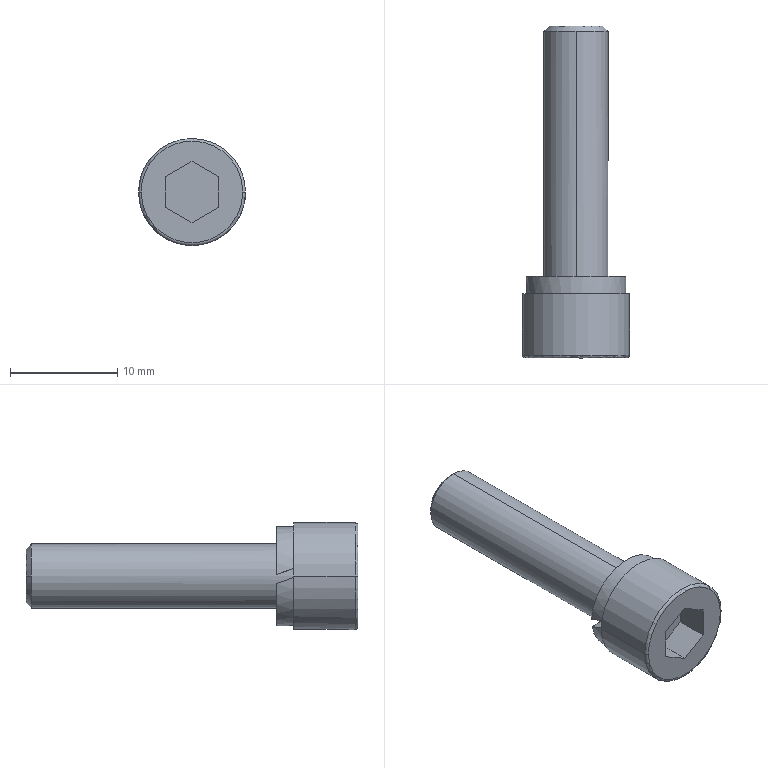Part | STEP file | Positioning_id2154_x_t | 1 solid | 25 faces | box 10 x 31 x 10 mm | volume 1171 mm3 | plane 13 | cylinder 8 | cone 2 | torus 2 | commonest cylinder face diameters 6 x2 6.1 x2 9.3 x2 10 x2